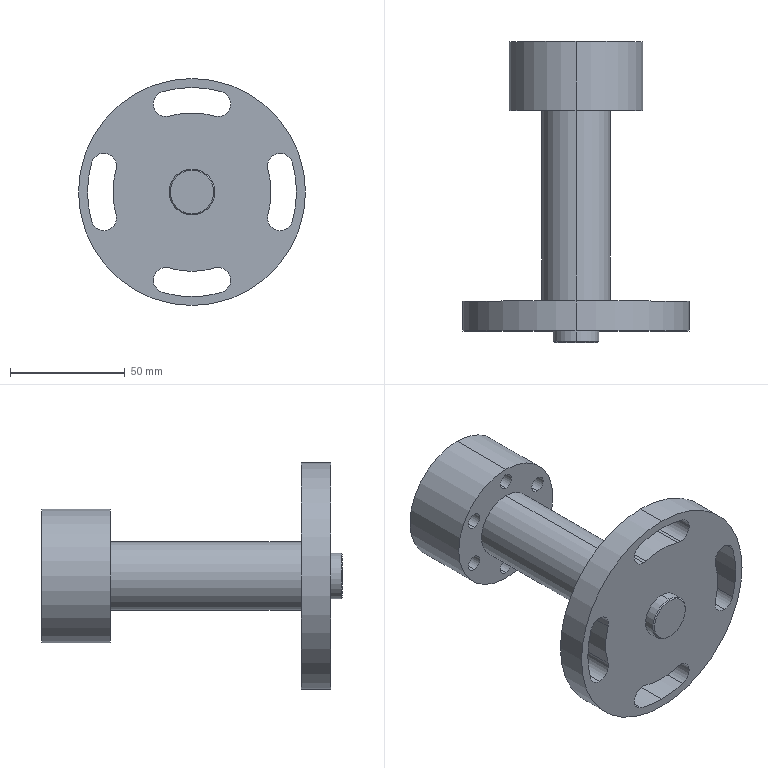Part | SolidWorks | features BaseBody 1 | 1 solid | 55 faces | box 98.8 x 131 x 98.8 mm | volume 207215 mm3 | cylinder 44 | cone 6 | plane 5 | commonest cylinder face diameters 7 x12 11 x12 69 x5 91 x5 20 x4 30 x2